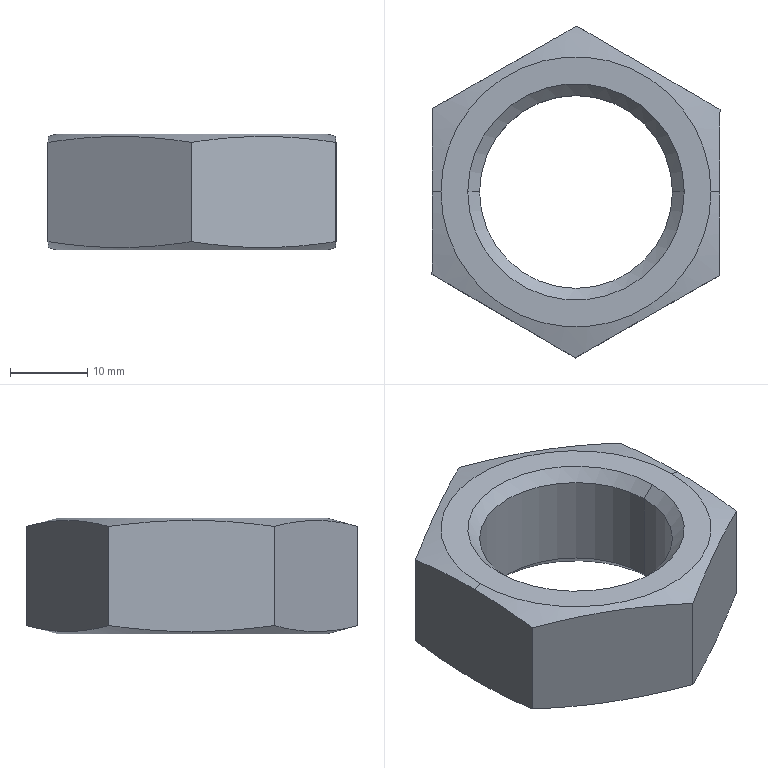Part | SolidWorks | features Cut 2, Chamfer 1, Extrusion 1 | 1 solid | 18 faces | box 37.323 x 43 x 15 mm | volume 10304 mm3 | cone 8 | plane 8 | cylinder 2 | commonest cylinder face diameters 25 x2
STEP:
#1=CARTESIAN_POINT('',(-12.5,0.,13.479));
#2=VERTEX_POINT('',#1);
#3=CARTESIAN_POINT('',(12.5,0.,13.479));
#4=VERTEX_POINT('',#3);
#5=CARTESIAN_POINT('',(0.,0.,13.479));
#6=DIRECTION('',(0.,0.,1.));
#7=DIRECTION('',(1.,0.,0.));
#8=AXIS2_PLACEMENT_3D('',#5,#6,#7);
#9=CIRCLE('',#8,12.5);
#10=EDGE_CURVE('',#2,#4,#9,.T.);
#11=ORIENTED_EDGE('',*,*,#10,.F.);
#12=CARTESIAN_POINT('',(-14.021,0.,15.));
#13=VERTEX_POINT('',#12);
#14=CARTESIAN_POINT('',(-12.5,0.,13.479));
#15=DIRECTION('',(-0.7071,0.,0.7071));
#16=VECTOR('',#15,1000.);
#17=LINE('',#14,#16);
#18=EDGE_CURVE('',#2,#13,#17,.T.);
#19=ORIENTED_EDGE('',*,*,#18,.T.);
#20=CARTESIAN_POINT('',(14.021,0.,15.));
#21=VERTEX_POINT('',#20);
#22=CARTESIAN_POINT('',(0.,0.,15.));
#23=DIRECTION('',(0.,0.,-1.));
#24=DIRECTION('',(1.,0.,0.));
#25=AXIS2_PLACEMENT_3D('',#22,#23,#24);
#26=CIRCLE('',#25,14.021);
#27=EDGE_CURVE('',#21,#13,#26,.T.);
#28=ORIENTED_EDGE('',*,*,#27,.F.);
#29=CARTESIAN_POINT('',(12.5,0.,13.479));
#30=DIRECTION('',(0.7071,0.,0.7071));
#31=VECTOR('',#30,1000.);
#32=LINE('',#29,#31);
#33=EDGE_CURVE('',#4,#21,#32,.T.);
#34=ORIENTED_EDGE('',*,*,#33,.F.);
#35=EDGE_LOOP('',(#11,#19,#28,#34));
#36=FACE_OUTER_BOUND('',#35,.T.);
#37=CARTESIAN_POINT('',(0.,0.,13.479));
#38=DIRECTION('',(0.,0.,1.));
#39=DIRECTION('',(1.,0.,0.));
#40=AXIS2_PLACEMENT_3D('',#37,#38,#39);
#41=CONICAL_SURFACE('',#40,12.5,0.7854);
#42=ADVANCED_FACE('',(#36),#41,.F.);
#43=CARTESIAN_POINT('',(12.5,0.,1.521));
#44=VERTEX_POINT('',#43);
#45=CARTESIAN_POINT('',(-12.5,0.,1.521));
#46=VERTEX_POINT('',#45);
#47=CARTESIAN_POINT('',(0.,0.,1.521));
#48=DIRECTION('',(0.,0.,-1.));
#49=DIRECTION('',(1.,0.,0.));
#50=AXIS2_PLACEMENT_3D('',#47,#48,#49);
#51=CIRCLE('',#50,12.5);
#52=EDGE_CURVE('',#44,#46,#51,.T.);
#53=ORIENTED_EDGE('',*,*,#52,.F.);
#54=CARTESIAN_POINT('',(14.021,0.,0.));
#55=VERTEX_POINT('',#54);
#56=CARTESIAN_POINT('',(14.021,0.,0.));
#57=DIRECTION('',(0.7071,0.,-0.7071));
#58=VECTOR('',#57,1000.);
#59=LINE('',#56,#58);
#60=EDGE_CURVE('',#44,#55,#59,.T.);
#61=ORIENTED_EDGE('',*,*,#60,.T.);
#62=CARTESIAN_POINT('',(-14.021,0.,0.));
#63=VERTEX_POINT('',#62);
#64=CARTESIAN_POINT('',(0.,0.,0.));
#65=DIRECTION('',(0.,0.,1.));
#66=DIRECTION('',(1.,0.,0.));
#67=AXIS2_PLACEMENT_3D('',#64,#65,#66);
#68=CIRCLE('',#67,14.021);
#69=EDGE_CURVE('',#63,#55,#68,.T.);
#70=ORIENTED_EDGE('',*,*,#69,.F.);
#71=CARTESIAN_POINT('',(-14.021,0.,0.));
#72=DIRECTION('',(-0.7071,0.,-0.7071));
#73=VECTOR('',#72,1000.);
#74=LINE('',#71,#73);
#75=EDGE_CURVE('',#46,#63,#74,.T.);
#76=ORIENTED_EDGE('',*,*,#75,.F.);
#77=EDGE_LOOP('',(#53,#61,#70,#76));
#78=FACE_OUTER_BOUND('',#77,.T.);
#79=CARTESIAN_POINT('',(0.,0.,0.));
#80=DIRECTION('',(0.,0.,-1.));
#81=DIRECTION('',(-1.,0.,0.));
#82=AXIS2_PLACEMENT_3D('',#79,#80,#81);
#83=CONICAL_SURFACE('',#82,14.021,0.7854);
#84=ADVANCED_FACE('',(#78),#83,.F.);
#85=CARTESIAN_POINT('',(-17.5,0.,15.));
#86=VERTEX_POINT('',#85);
#87=CARTESIAN_POINT('',(17.5,0.,15.));
#88=VERTEX_POINT('',#87);
#89=CARTESIAN_POINT('',(0.,0.,15.));
#90=DIRECTION('',(0.,0.,1.));
#91=DIRECTION('',(1.,0.,0.));
#92=AXIS2_PLACEMENT_3D('',#89,#90,#91);
#93=CIRCLE('',#92,17.5);
#94=EDGE_CURVE('',#86,#88,#93,.T.);
#95=ORIENTED_EDGE('',*,*,#94,.F.);
#96=CARTESIAN_POINT('',(-18.62,0.,14.7));
#97=VERTEX_POINT('',#96);
#98=CARTESIAN_POINT('',(-17.5,0.,15.));
#99=DIRECTION('',(-0.9659,0.,-0.2588));
#100=VECTOR('',#99,1000.);
#101=LINE('',#98,#100);
#102=EDGE_CURVE('',#86,#97,#101,.T.);
#103=ORIENTED_EDGE('',*,*,#102,.T.);
#104=CARTESIAN_POINT('',(-18.662,-10.677,13.928));
#105=VERTEX_POINT('',#104);
#106=CARTESIAN_POINT('',(-18.62,0.,14.7));
#107=CARTESIAN_POINT('',(-18.627,-1.779,14.698));
#108=CARTESIAN_POINT('',(-18.634,-3.559,14.627));
#109=CARTESIAN_POINT('',(-18.648,-7.118,14.36));
#110=CARTESIAN_POINT('',(-18.655,-8.897,14.167));
#111=CARTESIAN_POINT('',(-18.662,-10.677,13.928));
#112=B_SPLINE_CURVE_WITH_KNOTS('',3,(#106,#107,#108,#109,#110,#111),.UNSPECIFIED.,.F.,.F.,(4,2,4),(0.01082,0.01616,0.0215),.UNSPECIFIED.);
#113=EDGE_CURVE('',#97,#105,#112,.T.);
#114=ORIENTED_EDGE('',*,*,#113,.T.);
#115=CARTESIAN_POINT('',(-0.08457,-21.5,13.928));
#116=VERTEX_POINT('',#115);
#117=CARTESIAN_POINT('',(-18.662,-10.677,13.928));
#118=CARTESIAN_POINT('',(-17.114,-11.579,14.168));
#119=CARTESIAN_POINT('',(-15.566,-12.481,14.363));
#120=CARTESIAN_POINT('',(-12.469,-14.284,14.629));
#121=CARTESIAN_POINT('',(-9.373,-16.088,14.771));
#122=CARTESIAN_POINT('',(-6.277,-17.892,14.629));
#123=CARTESIAN_POINT('',(-3.181,-19.696,14.363));
#124=CARTESIAN_POINT('',(-1.633,-20.598,14.168));
#125=CARTESIAN_POINT('',(-0.08457,-21.5,13.928));
#126=B_SPLINE_CURVE_WITH_KNOTS('',3,(#117,#118,#119,#120,#121,#122,#123,#124,#125),.UNSPECIFIED.,.F.,.F.,(4,2,1,2,4),(0.000000232,0.005375,0.01075,0.01613,0.0215),.UNSPECIFIED.);
#127=EDGE_CURVE('',#105,#116,#126,.T.);
#128=ORIENTED_EDGE('',*,*,#127,.T.);
#129=CARTESIAN_POINT('',(18.577,-10.823,13.928));
#130=VERTEX_POINT('',#129);
#131=CARTESIAN_POINT('',(-0.08457,-21.5,13.928));
#132=CARTESIAN_POINT('',(1.471,-20.61,14.168));
#133=CARTESIAN_POINT('',(3.026,-19.72,14.363));
#134=CARTESIAN_POINT('',(6.136,-17.941,14.629));
#135=CARTESIAN_POINT('',(9.246,-16.161,14.771));
#136=CARTESIAN_POINT('',(12.357,-14.382,14.629));
#137=CARTESIAN_POINT('',(15.467,-12.603,14.363));
#138=CARTESIAN_POINT('',(17.022,-11.713,14.168));
#139=CARTESIAN_POINT('',(18.577,-10.823,13.928));
#140=B_SPLINE_CURVE_WITH_KNOTS('',3,(#131,#132,#133,#134,#135,#136,#137,#138,#139),.UNSPECIFIED.,.F.,.F.,(4,2,1,2,4),(0.00000023,0.005375,0.01075,0.01613,0.0215),.UNSPECIFIED.);
#141=EDGE_CURVE('',#116,#130,#140,.T.);
#142=ORIENTED_EDGE('',*,*,#141,.T.);
#143=CARTESIAN_POINT('',(18.62,0.,14.7));
#144=VERTEX_POINT('',#143);
#145=CARTESIAN_POINT('',(18.577,-10.823,13.928));
#146=CARTESIAN_POINT('',(18.584,-9.019,14.17));
#147=CARTESIAN_POINT('',(18.591,-7.215,14.366));
#148=CARTESIAN_POINT('',(18.605,-3.608,14.632));
#149=CARTESIAN_POINT('',(18.613,-1.804,14.702));
#150=CARTESIAN_POINT('',(18.62,0.,14.7));
#151=B_SPLINE_CURVE_WITH_KNOTS('',3,(#145,#146,#147,#148,#149,#150),.UNSPECIFIED.,.F.,.F.,(4,2,4),(0.0000002,0.005412,0.01082),.UNSPECIFIED.);
#152=EDGE_CURVE('',#130,#144,#151,.T.);
#153=ORIENTED_EDGE('',*,*,#152,.T.);
#154=CARTESIAN_POINT('',(17.5,0.,15.));
#155=DIRECTION('',(0.9659,0.,-0.2588));
#156=VECTOR('',#155,1000.);
#157=LINE('',#154,#156);
#158=EDGE_CURVE('',#88,#144,#157,.T.);
#159=ORIENTED_EDGE('',*,*,#158,.F.);
#160=EDGE_LOOP('',(#95,#103,#114,#128,#142,#153,#159));
#161=FACE_OUTER_BOUND('',#160,.T.);
#162=CARTESIAN_POINT('',(0.,0.,15.));
#163=DIRECTION('',(0.,0.,-1.));
#164=DIRECTION('',(1.,0.,0.));
#165=AXIS2_PLACEMENT_3D('',#162,#163,#164);
#166=CONICAL_SURFACE('',#165,17.5,1.309);
#167=ADVANCED_FACE('',(#161),#166,.T.);
#168=CARTESIAN_POINT('',(17.5,0.,0.));
#169=VERTEX_POINT('',#168);
#170=CARTESIAN_POINT('',(-17.5,0.,0.));
#171=VERTEX_POINT('',#170);
#172=CARTESIAN_POINT('',(0.,0.,0.));
#173=DIRECTION('',(0.,0.,-1.));
#174=DIRECTION('',(-1.,0.,0.));
#175=AXIS2_PLACEMENT_3D('',#172,#173,#174);
#176=CIRCLE('',#175,17.5);
#177=EDGE_CURVE('',#169,#171,#176,.T.);
#178=ORIENTED_EDGE('',*,*,#177,.F.);
#179=CARTESIAN_POINT('',(18.62,0.,0.3));
#180=VERTEX_POINT('',#179);
#181=CARTESIAN_POINT('',(17.5,0.,0.));
#182=DIRECTION('',(0.9659,0.,0.2588));
#183=VECTOR('',#182,1000.);
#184=LINE('',#181,#183);
#185=EDGE_CURVE('',#169,#180,#184,.T.);
#186=ORIENTED_EDGE('',*,*,#185,.T.);
#187=CARTESIAN_POINT('',(18.577,-10.823,1.072));
#188=VERTEX_POINT('',#187);
#189=CARTESIAN_POINT('',(18.62,0.,0.3));
#190=CARTESIAN_POINT('',(18.613,-1.804,0.2981));
#191=CARTESIAN_POINT('',(18.605,-3.608,0.3678));
#192=CARTESIAN_POINT('',(18.591,-7.215,0.6342));
#193=CARTESIAN_POINT('',(18.584,-9.019,0.8301));
#194=CARTESIAN_POINT('',(18.577,-10.823,1.072));
#195=B_SPLINE_CURVE_WITH_KNOTS('',3,(#189,#190,#191,#192,#193,#194),.UNSPECIFIED.,.F.,.F.,(4,2,4),(0.01068,0.01609,0.0215),.UNSPECIFIED.);
#196=EDGE_CURVE('',#180,#188,#195,.T.);
#197=ORIENTED_EDGE('',*,*,#196,.T.);
#198=CARTESIAN_POINT('',(-0.08457,-21.5,1.072));
#199=VERTEX_POINT('',#198);
#200=CARTESIAN_POINT('',(18.577,-10.823,1.072));
#201=CARTESIAN_POINT('',(17.022,-11.713,0.8318));
#202=CARTESIAN_POINT('',(15.467,-12.603,0.6369));
#203=CARTESIAN_POINT('',(12.357,-14.382,0.3706));
#204=CARTESIAN_POINT('',(9.246,-16.161,0.2294));
#205=CARTESIAN_POINT('',(6.136,-17.941,0.3706));
#206=CARTESIAN_POINT('',(3.026,-19.72,0.6369));
#207=CARTESIAN_POINT('',(1.471,-20.61,0.8318));
#208=CARTESIAN_POINT('',(-0.08457,-21.5,1.072));
#209=B_SPLINE_CURVE_WITH_KNOTS('',3,(#200,#201,#202,#203,#204,#205,#206,#207,#208),.UNSPECIFIED.,.F.,.F.,(4,2,1,2,4),(0.00000023,0.005375,0.01075,0.01613,0.0215),.UNSPECIFIED.);
#210=EDGE_CURVE('',#188,#199,#209,.T.);
#211=ORIENTED_EDGE('',*,*,#210,.T.);
#212=CARTESIAN_POINT('',(-18.662,-10.677,1.072));
#213=VERTEX_POINT('',#212);
#214=CARTESIAN_POINT('',(-0.08457,-21.5,1.072));
#215=CARTESIAN_POINT('',(-1.633,-20.598,0.8318));
#216=CARTESIAN_POINT('',(-3.181,-19.696,0.6369));
#217=CARTESIAN_POINT('',(-6.277,-17.892,0.3706));
#218=CARTESIAN_POINT('',(-9.373,-16.088,0.2294));
#219=CARTESIAN_POINT('',(-12.469,-14.284,0.3706));
#220=CARTESIAN_POINT('',(-15.566,-12.481,0.6369));
#221=CARTESIAN_POINT('',(-17.114,-11.579,0.8318));
#222=CARTESIAN_POINT('',(-18.662,-10.677,1.072));
#223=B_SPLINE_CURVE_WITH_KNOTS('',3,(#214,#215,#216,#217,#218,#219,#220,#221,#222),.UNSPECIFIED.,.F.,.F.,(4,2,1,2,4),(0.000000232,0.005375,0.01075,0.01613,0.0215),.UNSPECIFIED.);
#224=EDGE_CURVE('',#199,#213,#223,.T.);
#225=ORIENTED_EDGE('',*,*,#224,.T.);
#226=CARTESIAN_POINT('',(-18.62,0.,0.3));
#227=VERTEX_POINT('',#226);
#228=CARTESIAN_POINT('',(-18.662,-10.677,1.072));
#229=CARTESIAN_POINT('',(-18.655,-8.897,0.8334));
#230=CARTESIAN_POINT('',(-18.648,-7.118,0.6395));
#231=CARTESIAN_POINT('',(-18.634,-3.559,0.3734));
#232=CARTESIAN_POINT('',(-18.627,-1.779,0.3019));
#233=CARTESIAN_POINT('',(-18.62,0.,0.3));
#234=B_SPLINE_CURVE_WITH_KNOTS('',3,(#228,#229,#230,#231,#232,#233),.UNSPECIFIED.,.F.,.F.,(4,2,4),(0.0000002,0.005339,0.01068),.UNSPECIFIED.);
#235=EDGE_CURVE('',#213,#227,#234,.T.);
#236=ORIENTED_EDGE('',*,*,#235,.T.);
#237=CARTESIAN_POINT('',(-17.5,0.,0.));
#238=DIRECTION('',(-0.9659,0.,0.2588));
#239=VECTOR('',#238,1000.);
#240=LINE('',#237,#239);
#241=EDGE_CURVE('',#171,#227,#240,.T.);
#242=ORIENTED_EDGE('',*,*,#241,.F.);
#243=EDGE_LOOP('',(#178,#186,#197,#211,#225,#236,#242));
#244=FACE_OUTER_BOUND('',#243,.T.);
#245=CARTESIAN_POINT('',(0.,0.,0.));
#246=DIRECTION('',(0.,0.,1.));
#247=DIRECTION('',(-1.,0.,0.));
#248=AXIS2_PLACEMENT_3D('',#245,#246,#247);
#249=CONICAL_SURFACE('',#248,17.5,1.309);
#250=ADVANCED_FACE('',(#244),#249,.T.);
#251=ORIENTED_EDGE('',*,*,#10,.T.);
#252=CARTESIAN_POINT('',(12.5,0.,15.));
#253=DIRECTION('',(0.,0.,-1.));
#254=VECTOR('',#253,1000.);
#255=LINE('',#252,#254);
#256=EDGE_CURVE('',#4,#44,#255,.T.);
#257=ORIENTED_EDGE('',*,*,#256,.T.);
#258=ORIENTED_EDGE('',*,*,#52,.T.);
#259=CARTESIAN_POINT('',(-12.5,0.,15.));
#260=DIRECTION('',(0.,0.,-1.));
#261=VECTOR('',#260,1000.);
#262=LINE('',#259,#261);
#263=EDGE_CURVE('',#2,#46,#262,.T.);
#264=ORIENTED_EDGE('',*,*,#263,.F.);
#265=EDGE_LOOP('',(#251,#257,#258,#264));
#266=FACE_OUTER_BOUND('',#265,.T.);
#267=CARTESIAN_POINT('',(0.,0.,15.));
#268=DIRECTION('',(0.,0.,-1.));
#269=DIRECTION('',(-1.,0.,0.));
#270=AXIS2_PLACEMENT_3D('',#267,#268,#269);
#271=CYLINDRICAL_SURFACE('',#270,12.5);
#272=ADVANCED_FACE('',(#266),#271,.F.);
#273=CARTESIAN_POINT('',(18.662,10.677,13.928));
#274=VERTEX_POINT('',#273);
#275=CARTESIAN_POINT('',(0.08457,21.5,13.928));
#276=VERTEX_POINT('',#275);
#277=CARTESIAN_POINT('',(18.662,10.677,13.928));
#278=CARTESIAN_POINT('',(17.114,11.579,14.168));
#279=CARTESIAN_POINT('',(15.566,12.481,14.363));
#280=CARTESIAN_POINT('',(12.469,14.284,14.629));
#281=CARTESIAN_POINT('',(9.373,16.088,14.771));
#282=CARTESIAN_POINT('',(6.277,17.892,14.629));
#283=CARTESIAN_POINT('',(3.181,19.696,14.363));
#284=CARTESIAN_POINT('',(1.633,20.598,14.168));
#285=CARTESIAN_POINT('',(0.08457,21.5,13.928));
#286=B_SPLINE_CURVE_WITH_KNOTS('',3,(#277,#278,#279,#280,#281,#282,#283,#284,#285),.UNSPECIFIED.,.F.,.F.,(4,2,1,2,4),(0.000000232,0.005375,0.01075,0.01613,0.0215),.UNSPECIFIED.);
#287=EDGE_CURVE('',#274,#276,#286,.T.);
#288=ORIENTED_EDGE('',*,*,#287,.F.);
#289=CARTESIAN_POINT('',(18.662,10.677,1.072));
#290=VERTEX_POINT('',#289);
#291=CARTESIAN_POINT('',(18.662,10.677,15.));
#292=DIRECTION('',(0.,0.,-1.));
#293=VECTOR('',#292,1000.);
#294=LINE('',#291,#293);
#295=EDGE_CURVE('',#274,#290,#294,.T.);
#296=ORIENTED_EDGE('',*,*,#295,.T.);
#297=CARTESIAN_POINT('',(0.08457,21.5,1.072));
#298=VERTEX_POINT('',#297);
#299=CARTESIAN_POINT('',(0.08457,21.5,1.072));
#300=CARTESIAN_POINT('',(1.633,20.598,0.8318));
#301=CARTESIAN_POINT('',(3.181,19.696,0.6369));
#302=CARTESIAN_POINT('',(6.277,17.892,0.3706));
#303=CARTESIAN_POINT('',(9.373,16.088,0.2294));
#304=CARTESIAN_POINT('',(12.469,14.284,0.3706));
#305=CARTESIAN_POINT('',(15.566,12.481,0.6369));
#306=CARTESIAN_POINT('',(17.114,11.579,0.8318));
#307=CARTESIAN_POINT('',(18.662,10.677,1.072));
#308=B_SPLINE_CURVE_WITH_KNOTS('',3,(#299,#300,#301,#302,#303,#304,#305,#306,#307),.UNSPECIFIED.,.F.,.F.,(4,2,1,2,4),(0.000000232,0.005375,0.01075,0.01613,0.0215),.UNSPECIFIED.);
#309=EDGE_CURVE('',#298,#290,#308,.T.);
#310=ORIENTED_EDGE('',*,*,#309,.F.);
#311=CARTESIAN_POINT('',(0.08457,21.5,15.));
#312=DIRECTION('',(0.,0.,-1.));
#313=VECTOR('',#312,1000.);
#314=LINE('',#311,#313);
#315=EDGE_CURVE('',#276,#298,#314,.T.);
#316=ORIENTED_EDGE('',*,*,#315,.F.);
#317=EDGE_LOOP('',(#288,#296,#310,#316));
#318=FACE_OUTER_BOUND('',#317,.T.);
#319=CARTESIAN_POINT('',(18.662,10.677,15.));
#320=DIRECTION('',(-0.5034,-0.8641,0.));
#321=DIRECTION('',(0.8641,-0.5034,0.));
#322=AXIS2_PLACEMENT_3D('',#319,#320,#321);
#323=PLANE('',#322);
#324=ADVANCED_FACE('',(#318),#323,.F.);
#325=CARTESIAN_POINT('',(-18.577,10.823,13.928));
#326=VERTEX_POINT('',#325);
#327=CARTESIAN_POINT('',(0.08457,21.5,13.928));
#328=CARTESIAN_POINT('',(-1.471,20.61,14.168));
#329=CARTESIAN_POINT('',(-3.026,19.72,14.363));
#330=CARTESIAN_POINT('',(-6.136,17.941,14.629));
#331=CARTESIAN_POINT('',(-9.246,16.161,14.771));
#332=CARTESIAN_POINT('',(-12.357,14.382,14.629));
#333=CARTESIAN_POINT('',(-15.467,12.603,14.363));
#334=CARTESIAN_POINT('',(-17.022,11.713,14.168));
#335=CARTESIAN_POINT('',(-18.577,10.823,13.928));
#336=B_SPLINE_CURVE_WITH_KNOTS('',3,(#327,#328,#329,#330,#331,#332,#333,#334,#335),.UNSPECIFIED.,.F.,.F.,(4,2,1,2,4),(0.00000023,0.005375,0.01075,0.01613,0.0215),.UNSPECIFIED.);
#337=EDGE_CURVE('',#276,#326,#336,.T.);
#338=ORIENTED_EDGE('',*,*,#337,.F.);
#339=ORIENTED_EDGE('',*,*,#315,.T.);
#340=CARTESIAN_POINT('',(-18.577,10.823,1.072));
#341=VERTEX_POINT('',#340);
#342=CARTESIAN_POINT('',(-18.577,10.823,1.072));
#343=CARTESIAN_POINT('',(-17.022,11.713,0.8318));
#344=CARTESIAN_POINT('',(-15.467,12.603,0.6369));
#345=CARTESIAN_POINT('',(-12.357,14.382,0.3706));
#346=CARTESIAN_POINT('',(-9.246,16.161,0.2294));
#347=CARTESIAN_POINT('',(-6.136,17.941,0.3706));
#348=CARTESIAN_POINT('',(-3.026,19.72,0.6369));
#349=CARTESIAN_POINT('',(-1.471,20.61,0.8318));
#350=CARTESIAN_POINT('',(0.08457,21.5,1.072));
#351=B_SPLINE_CURVE_WITH_KNOTS('',3,(#342,#343,#344,#345,#346,#347,#348,#349,#350),.UNSPECIFIED.,.F.,.F.,(4,2,1,2,4),(0.00000023,0.005375,0.01075,0.01613,0.0215),.UNSPECIFIED.);
#352=EDGE_CURVE('',#341,#298,#351,.T.);
#353=ORIENTED_EDGE('',*,*,#352,.F.);
#354=CARTESIAN_POINT('',(-18.577,10.823,15.));
#355=DIRECTION('',(0.,0.,-1.));
#356=VECTOR('',#355,1000.);
#357=LINE('',#354,#356);
#358=EDGE_CURVE('',#326,#341,#357,.T.);
#359=ORIENTED_EDGE('',*,*,#358,.F.);
#360=EDGE_LOOP('',(#338,#339,#353,#359));
#361=FACE_OUTER_BOUND('',#360,.T.);
#362=CARTESIAN_POINT('',(0.08457,21.5,15.));
#363=DIRECTION('',(0.4966,-0.868,0.));
#364=DIRECTION('',(0.868,0.4966,0.));
#365=AXIS2_PLACEMENT_3D('',#362,#363,#364);
#366=PLANE('',#365);
#367=ADVANCED_FACE('',(#361),#366,.F.);
#368=CARTESIAN_POINT('',(-18.577,10.823,13.928));
#369=CARTESIAN_POINT('',(-18.584,9.019,14.17));
#370=CARTESIAN_POINT('',(-18.591,7.215,14.366));
#371=CARTESIAN_POINT('',(-18.605,3.608,14.632));
#372=CARTESIAN_POINT('',(-18.613,1.804,14.702));
#373=CARTESIAN_POINT('',(-18.62,0.,14.7));
#374=B_SPLINE_CURVE_WITH_KNOTS('',3,(#368,#369,#370,#371,#372,#373),.UNSPECIFIED.,.F.,.F.,(4,2,4),(0.0000002,0.005412,0.01082),.UNSPECIFIED.);
#375=EDGE_CURVE('',#326,#97,#374,.T.);
#376=ORIENTED_EDGE('',*,*,#375,.F.);
#377=ORIENTED_EDGE('',*,*,#358,.T.);
#378=CARTESIAN_POINT('',(-18.62,0.,0.3));
#379=CARTESIAN_POINT('',(-18.613,1.804,0.2981));
#380=CARTESIAN_POINT('',(-18.605,3.608,0.3678));
#381=CARTESIAN_POINT('',(-18.591,7.215,0.6342));
#382=CARTESIAN_POINT('',(-18.584,9.019,0.8301));
#383=CARTESIAN_POINT('',(-18.577,10.823,1.072));
#384=B_SPLINE_CURVE_WITH_KNOTS('',3,(#378,#379,#380,#381,#382,#383),.UNSPECIFIED.,.F.,.F.,(4,2,4),(0.01068,0.01609,0.0215),.UNSPECIFIED.);
#385=EDGE_CURVE('',#227,#341,#384,.T.);
#386=ORIENTED_EDGE('',*,*,#385,.F.);
#387=ORIENTED_EDGE('',*,*,#235,.F.);
#388=CARTESIAN_POINT('',(-18.662,-10.677,15.));
#389=DIRECTION('',(0.,0.,-1.));
#390=VECTOR('',#389,1000.);
#391=LINE('',#388,#390);
#392=EDGE_CURVE('',#105,#213,#391,.T.);
#393=ORIENTED_EDGE('',*,*,#392,.F.);
#394=ORIENTED_EDGE('',*,*,#113,.F.);
#395=EDGE_LOOP('',(#376,#377,#386,#387,#393,#394));
#396=FACE_OUTER_BOUND('',#395,.T.);
#397=CARTESIAN_POINT('',(-18.577,10.823,15.));
#398=DIRECTION('',(1.,-0.003934,0.));
#399=DIRECTION('',(0.003934,1.,0.));
#400=AXIS2_PLACEMENT_3D('',#397,#398,#399);
#401=PLANE('',#400);
#402=ADVANCED_FACE('',(#396),#401,.F.);
#403=ORIENTED_EDGE('',*,*,#127,.F.);
#404=ORIENTED_EDGE('',*,*,#392,.T.);
#405=ORIENTED_EDGE('',*,*,#224,.F.);
#406=CARTESIAN_POINT('',(-0.08457,-21.5,15.));
#407=DIRECTION('',(0.,0.,-1.));
#408=VECTOR('',#407,1000.);
#409=LINE('',#406,#408);
#410=EDGE_CURVE('',#116,#199,#409,.T.);
#411=ORIENTED_EDGE('',*,*,#410,.F.);
#412=EDGE_LOOP('',(#403,#404,#405,#411));
#413=FACE_OUTER_BOUND('',#412,.T.);
#414=CARTESIAN_POINT('',(-18.662,-10.677,15.));
#415=DIRECTION('',(0.5034,0.8641,0.));
#416=DIRECTION('',(-0.8641,0.5034,0.));
#417=AXIS2_PLACEMENT_3D('',#414,#415,#416);
#418=PLANE('',#417);
#419=ADVANCED_FACE('',(#413),#418,.F.);
#420=ORIENTED_EDGE('',*,*,#141,.F.);
#421=ORIENTED_EDGE('',*,*,#410,.T.);
#422=ORIENTED_EDGE('',*,*,#210,.F.);
#423=CARTESIAN_POINT('',(18.577,-10.823,15.));
#424=DIRECTION('',(0.,0.,-1.));
#425=VECTOR('',#424,1000.);
#426=LINE('',#423,#425);
#427=EDGE_CURVE('',#130,#188,#426,.T.);
#428=ORIENTED_EDGE('',*,*,#427,.F.);
#429=EDGE_LOOP('',(#420,#421,#422,#428));
#430=FACE_OUTER_BOUND('',#429,.T.);
#431=CARTESIAN_POINT('',(-0.08457,-21.5,15.));
#432=DIRECTION('',(-0.4966,0.868,0.));
#433=DIRECTION('',(-0.868,-0.4966,0.));
#434=AXIS2_PLACEMENT_3D('',#431,#432,#433);
#435=PLANE('',#434);
#436=ADVANCED_FACE('',(#430),#435,.F.);
#437=ORIENTED_EDGE('',*,*,#152,.F.);
#438=ORIENTED_EDGE('',*,*,#427,.T.);
#439=ORIENTED_EDGE('',*,*,#196,.F.);
#440=CARTESIAN_POINT('',(18.662,10.677,1.072));
#441=CARTESIAN_POINT('',(18.655,8.897,0.8334));
#442=CARTESIAN_POINT('',(18.648,7.118,0.6395));
#443=CARTESIAN_POINT('',(18.634,3.559,0.3734));
#444=CARTESIAN_POINT('',(18.627,1.779,0.3019));
#445=CARTESIAN_POINT('',(18.62,0.,0.3));
#446=B_SPLINE_CURVE_WITH_KNOTS('',3,(#440,#441,#442,#443,#444,#445),.UNSPECIFIED.,.F.,.F.,(4,2,4),(0.0000002,0.005339,0.01068),.UNSPECIFIED.);
#447=EDGE_CURVE('',#290,#180,#446,.T.);
#448=ORIENTED_EDGE('',*,*,#447,.F.);
#449=ORIENTED_EDGE('',*,*,#295,.F.);
#450=CARTESIAN_POINT('',(18.62,0.,14.7));
#451=CARTESIAN_POINT('',(18.627,1.779,14.698));
#452=CARTESIAN_POINT('',(18.634,3.559,14.627));
#453=CARTESIAN_POINT('',(18.648,7.118,14.36));
#454=CARTESIAN_POINT('',(18.655,8.897,14.167));
#455=CARTESIAN_POINT('',(18.662,10.677,13.928));
#456=B_SPLINE_CURVE_WITH_KNOTS('',3,(#450,#451,#452,#453,#454,#455),.UNSPECIFIED.,.F.,.F.,(4,2,4),(0.01082,0.01616,0.0215),.UNSPECIFIED.);
#457=EDGE_CURVE('',#144,#274,#456,.T.);
#458=ORIENTED_EDGE('',*,*,#457,.F.);
#459=EDGE_LOOP('',(#437,#438,#439,#448,#449,#458));
#460=FACE_OUTER_BOUND('',#459,.T.);
#461=CARTESIAN_POINT('',(18.577,-10.823,15.));
#462=DIRECTION('',(-1.,0.003934,0.));
#463=DIRECTION('',(-0.003934,-1.,0.));
#464=AXIS2_PLACEMENT_3D('',#461,#462,#463);
#465=PLANE('',#464);
#466=ADVANCED_FACE('',(#460),#465,.F.);
#467=ORIENTED_EDGE('',*,*,#27,.T.);
#468=CARTESIAN_POINT('',(0.,0.,15.));
#469=DIRECTION('',(0.,0.,-1.));
#470=DIRECTION('',(1.,0.,0.));
#471=AXIS2_PLACEMENT_3D('',#468,#469,#470);
#472=CIRCLE('',#471,14.021);
#473=EDGE_CURVE('',#13,#21,#472,.T.);
#474=ORIENTED_EDGE('',*,*,#473,.T.);
#475=EDGE_LOOP('',(#467,#474));
#476=FACE_BOUND('',#475,.T.);
#477=CARTESIAN_POINT('',(0.,0.,15.));
#478=DIRECTION('',(0.,0.,1.));
#479=DIRECTION('',(1.,0.,0.));
#480=AXIS2_PLACEMENT_3D('',#477,#478,#479);
#481=CIRCLE('',#480,17.5);
#482=EDGE_CURVE('',#88,#86,#481,.T.);
#483=ORIENTED_EDGE('',*,*,#482,.T.);
#484=ORIENTED_EDGE('',*,*,#94,.T.);
#485=EDGE_LOOP('',(#483,#484));
#486=FACE_OUTER_BOUND('',#485,.T.);
#487=CARTESIAN_POINT('',(0.08457,21.5,15.));
#488=DIRECTION('',(0.,0.,1.));
#489=DIRECTION('',(1.,0.,0.));
#490=AXIS2_PLACEMENT_3D('',#487,#488,#489);
#491=PLANE('',#490);
#492=ADVANCED_FACE('',(#476,#486),#491,.T.);
#493=ORIENTED_EDGE('',*,*,#69,.T.);
#494=CARTESIAN_POINT('',(0.,0.,0.));
#495=DIRECTION('',(0.,0.,1.));
#496=DIRECTION('',(1.,0.,0.));
#497=AXIS2_PLACEMENT_3D('',#494,#495,#496);
#498=CIRCLE('',#497,14.021);
#499=EDGE_CURVE('',#55,#63,#498,.T.);
#500=ORIENTED_EDGE('',*,*,#499,.T.);
#501=EDGE_LOOP('',(#493,#500));
#502=FACE_BOUND('',#501,.T.);
#503=CARTESIAN_POINT('',(0.,0.,0.));
#504=DIRECTION('',(0.,0.,-1.));
#505=DIRECTION('',(-1.,0.,0.));
#506=AXIS2_PLACEMENT_3D('',#503,#504,#505);
#507=CIRCLE('',#506,17.5);
#508=EDGE_CURVE('',#171,#169,#507,.T.);
#509=ORIENTED_EDGE('',*,*,#508,.T.);
#510=ORIENTED_EDGE('',*,*,#177,.T.);
#511=EDGE_LOOP('',(#509,#510));
#512=FACE_OUTER_BOUND('',#511,.T.);
#513=CARTESIAN_POINT('',(0.08457,21.5,0.));
#514=DIRECTION('',(0.,0.,1.));
#515=DIRECTION('',(1.,0.,0.));
#516=AXIS2_PLACEMENT_3D('',#513,#514,#515);
#517=PLANE('',#516);
#518=ADVANCED_FACE('',(#502,#512),#517,.F.);
#519=ORIENTED_EDGE('',*,*,#256,.F.);
#520=CARTESIAN_POINT('',(0.,0.,13.479));
#521=DIRECTION('',(0.,0.,1.));
#522=DIRECTION('',(1.,0.,0.));
#523=AXIS2_PLACEMENT_3D('',#520,#521,#522);
#524=CIRCLE('',#523,12.5);
#525=EDGE_CURVE('',#4,#2,#524,.T.);
#526=ORIENTED_EDGE('',*,*,#525,.T.);
#527=ORIENTED_EDGE('',*,*,#263,.T.);
#528=CARTESIAN_POINT('',(0.,0.,1.521));
#529=DIRECTION('',(0.,0.,-1.));
#530=DIRECTION('',(1.,0.,0.));
#531=AXIS2_PLACEMENT_3D('',#528,#529,#530);
#532=CIRCLE('',#531,12.5);
#533=EDGE_CURVE('',#46,#44,#532,.T.);
#534=ORIENTED_EDGE('',*,*,#533,.T.);
#535=EDGE_LOOP('',(#519,#526,#527,#534));
#536=FACE_OUTER_BOUND('',#535,.T.);
#537=CARTESIAN_POINT('',(0.,0.,15.));
#538=DIRECTION('',(0.,0.,-1.));
#539=DIRECTION('',(-1.,0.,0.));
#540=AXIS2_PLACEMENT_3D('',#537,#538,#539);
#541=CYLINDRICAL_SURFACE('',#540,12.5);
#542=ADVANCED_FACE('',(#536),#541,.F.);
#543=ORIENTED_EDGE('',*,*,#185,.F.);
#544=ORIENTED_EDGE('',*,*,#508,.F.);
#545=ORIENTED_EDGE('',*,*,#241,.T.);
#546=ORIENTED_EDGE('',*,*,#385,.T.);
#547=ORIENTED_EDGE('',*,*,#352,.T.);
#548=ORIENTED_EDGE('',*,*,#309,.T.);
#549=ORIENTED_EDGE('',*,*,#447,.T.);
#550=EDGE_LOOP('',(#543,#544,#545,#546,#547,#548,#549));
#551=FACE_OUTER_BOUND('',#550,.T.);
#552=CARTESIAN_POINT('',(0.,0.,0.));
#553=DIRECTION('',(0.,0.,1.));
#554=DIRECTION('',(-1.,0.,0.));
#555=AXIS2_PLACEMENT_3D('',#552,#553,#554);
#556=CONICAL_SURFACE('',#555,17.5,1.309);
#557=ADVANCED_FACE('',(#551),#556,.T.);
#558=ORIENTED_EDGE('',*,*,#102,.F.);
#559=ORIENTED_EDGE('',*,*,#482,.F.);
#560=ORIENTED_EDGE('',*,*,#158,.T.);
#561=ORIENTED_EDGE('',*,*,#457,.T.);
#562=ORIENTED_EDGE('',*,*,#287,.T.);
#563=ORIENTED_EDGE('',*,*,#337,.T.);
#564=ORIENTED_EDGE('',*,*,#375,.T.);
#565=EDGE_LOOP('',(#558,#559,#560,#561,#562,#563,#564));
#566=FACE_OUTER_BOUND('',#565,.T.);
#567=CARTESIAN_POINT('',(0.,0.,15.));
#568=DIRECTION('',(0.,0.,-1.));
#569=DIRECTION('',(1.,0.,0.));
#570=AXIS2_PLACEMENT_3D('',#567,#568,#569);
#571=CONICAL_SURFACE('',#570,17.5,1.309);
#572=ADVANCED_FACE('',(#566),#571,.T.);
#573=ORIENTED_EDGE('',*,*,#60,.F.);
#574=ORIENTED_EDGE('',*,*,#533,.F.);
#575=ORIENTED_EDGE('',*,*,#75,.T.);
#576=ORIENTED_EDGE('',*,*,#499,.F.);
#577=EDGE_LOOP('',(#573,#574,#575,#576));
#578=FACE_OUTER_BOUND('',#577,.T.);
#579=CARTESIAN_POINT('',(0.,0.,0.));
#580=DIRECTION('',(0.,0.,-1.));
#581=DIRECTION('',(-1.,0.,0.));
#582=AXIS2_PLACEMENT_3D('',#579,#580,#581);
#583=CONICAL_SURFACE('',#582,14.021,0.7854);
#584=ADVANCED_FACE('',(#578),#583,.F.);
#585=ORIENTED_EDGE('',*,*,#18,.F.);
#586=ORIENTED_EDGE('',*,*,#525,.F.);
#587=ORIENTED_EDGE('',*,*,#33,.T.);
#588=ORIENTED_EDGE('',*,*,#473,.F.);
#589=EDGE_LOOP('',(#585,#586,#587,#588));
#590=FACE_OUTER_BOUND('',#589,.T.);
#591=CARTESIAN_POINT('',(0.,0.,13.479));
#592=DIRECTION('',(0.,0.,1.));
#593=DIRECTION('',(1.,0.,0.));
#594=AXIS2_PLACEMENT_3D('',#591,#592,#593);
#595=CONICAL_SURFACE('',#594,12.5,0.7854);
#596=ADVANCED_FACE('',(#590),#595,.F.);
#597=CLOSED_SHELL('',(#42,#84,#167,#250,#272,#324,#367,#402,#419,#436,#466,#492,#518,#542,#557,#572,#584,#596));
#598=MANIFOLD_SOLID_BREP('',#597);
#599=CARTESIAN_POINT('',(0.,0.,0.));
#600=DIRECTION('',(0.,0.,1.));
#601=DIRECTION('',(1.,0.,0.));
#602=AXIS2_PLACEMENT_3D('',#599,#600,#601);
#603=(LENGTH_UNIT()NAMED_UNIT(*)SI_UNIT(.MILLI.,.METRE.));
#604=UNCERTAINTY_MEASURE_WITH_UNIT(LENGTH_MEASURE(0.00001),#603,'','');
#605=(NAMED_UNIT(*)PLANE_ANGLE_UNIT()SI_UNIT($,.RADIAN.));
#606=(NAMED_UNIT(*)SI_UNIT($,.STERADIAN.)SOLID_ANGLE_UNIT());
#607=(GEOMETRIC_REPRESENTATION_CONTEXT(3)GLOBAL_UNCERTAINTY_ASSIGNED_CONTEXT((#604))GLOBAL_UNIT_ASSIGNED_CONTEXT((#603,#605,#606))REPRESENTATION_CONTEXT('',''));
#608=ADVANCED_BREP_SHAPE_REPRESENTATION('',(#598,#602),#607);